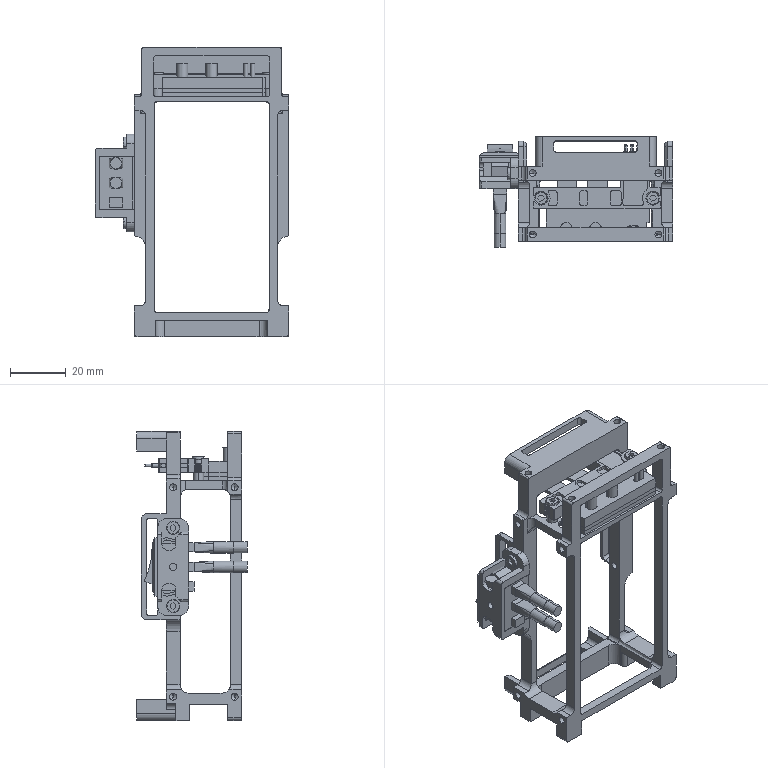Part | SolidWorks | features BaseBody 12 | 8 solids | 945 faces | box 69.4 x 39.5 x 103.5 mm | volume 27545 mm3 | plane 453 | cylinder 391 | cone 43 | spline 26 | torus 24 | sphere 8 | commonest cylinder face diameters 2.5 x86 3 x80 2 x72 4 x30 1.5 x20 0.4 x16